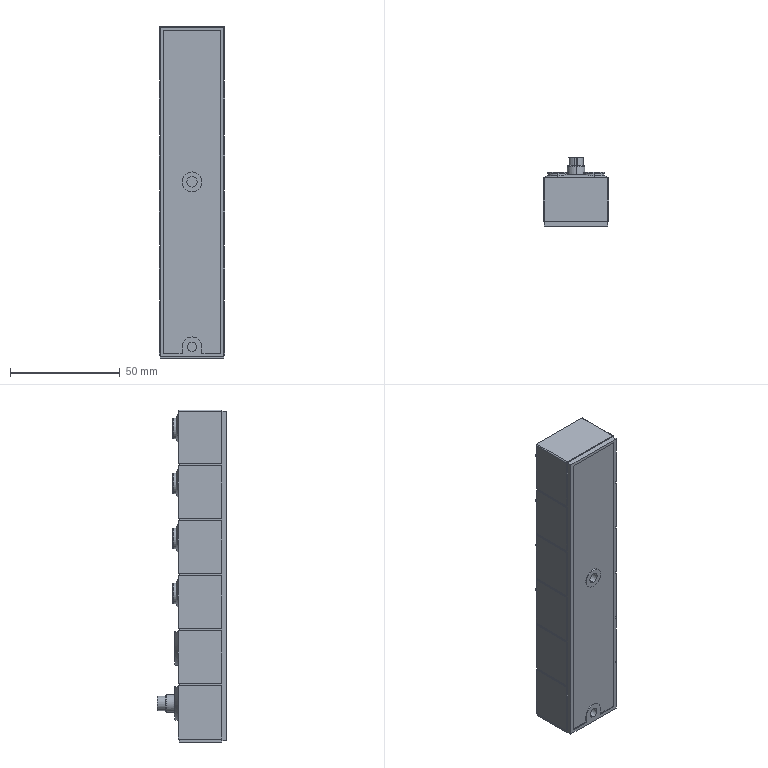Part | SolidWorks | features BaseBody 1 | 1 solid | 363 faces | box 30 x 31.5 x 151 mm | volume 97801 mm3 | plane 163 | cylinder 150 | spline 26 | cone 24 | commonest cylinder face diameters 1 x62 6 x18 9.34 x16 1.1 x10 7.188 x10 7.459 x8